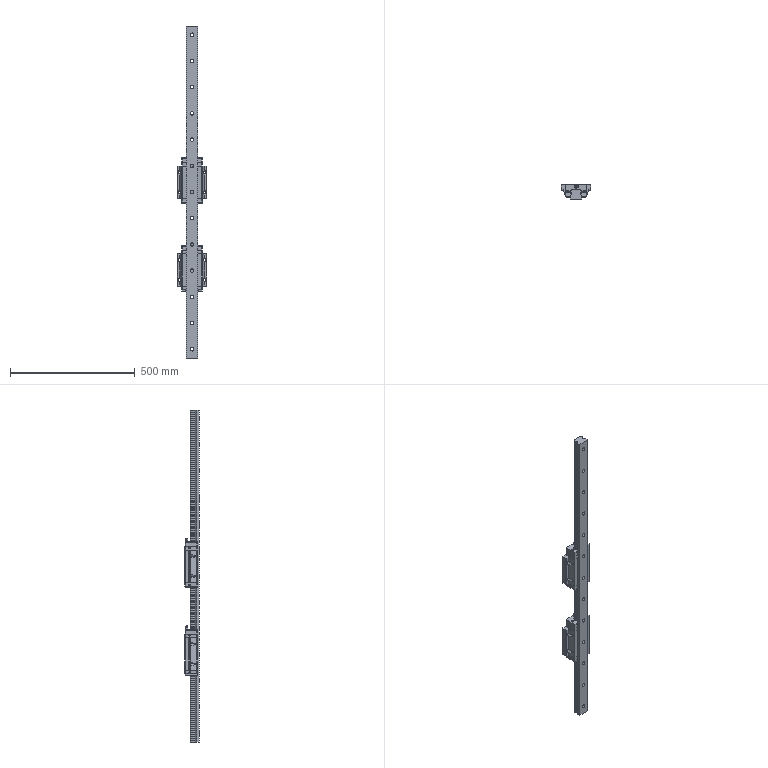Part | SolidWorks | features LocalLPattern 1, ReferencePattern 1 | 15 solids | 1041 faces | box 120 x 60 x 1330 mm | volume 3294670 mm3 | plane 679 | cylinder 246 | torus 50 | cone 46 | sphere 20 | commonest cylinder face diameters 3.924 x72 14 x26 20 x26 6.06 x24 0.818 x16 6.384 x16